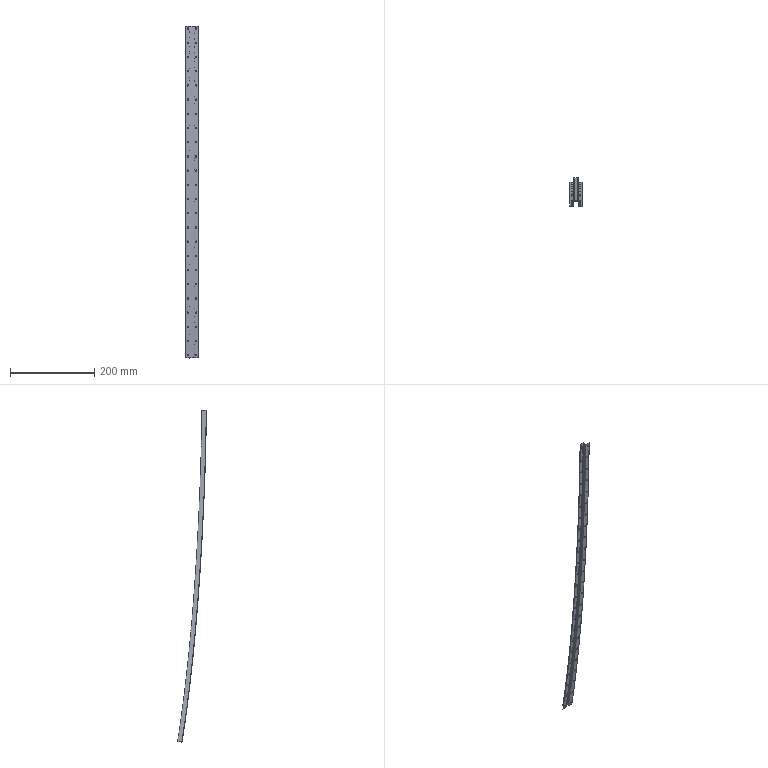Part | SolidWorks | features BaseBody 1 | 1 solid | 102 faces | box 30 x 68.6 x 788 mm | volume 10096 mm3 | cylinder 96 | plane 4 | spline 2 | commonest cylinder face diameters 3.2 x96